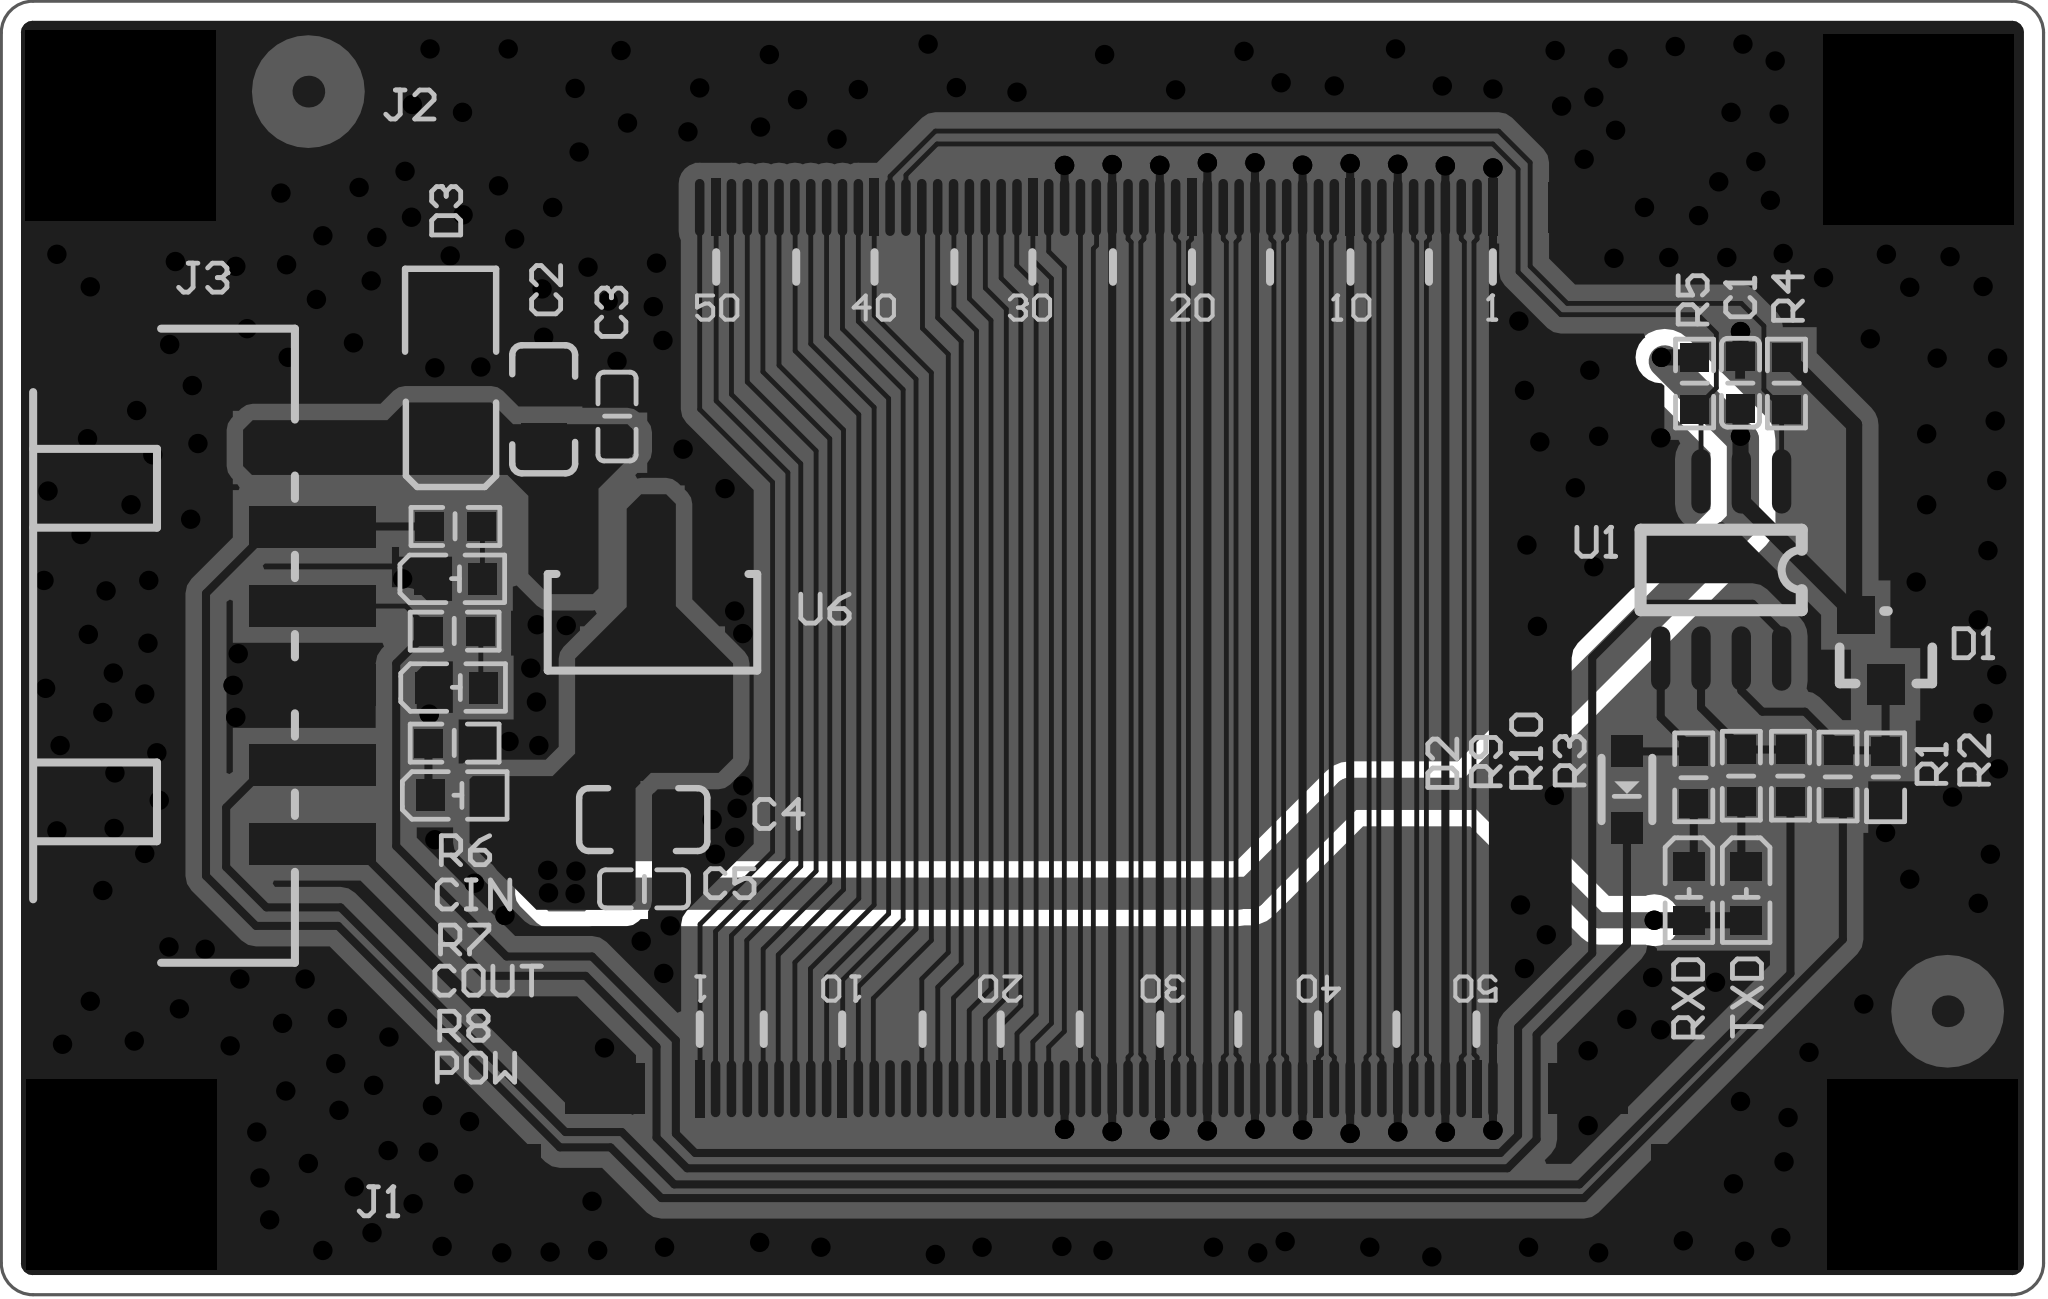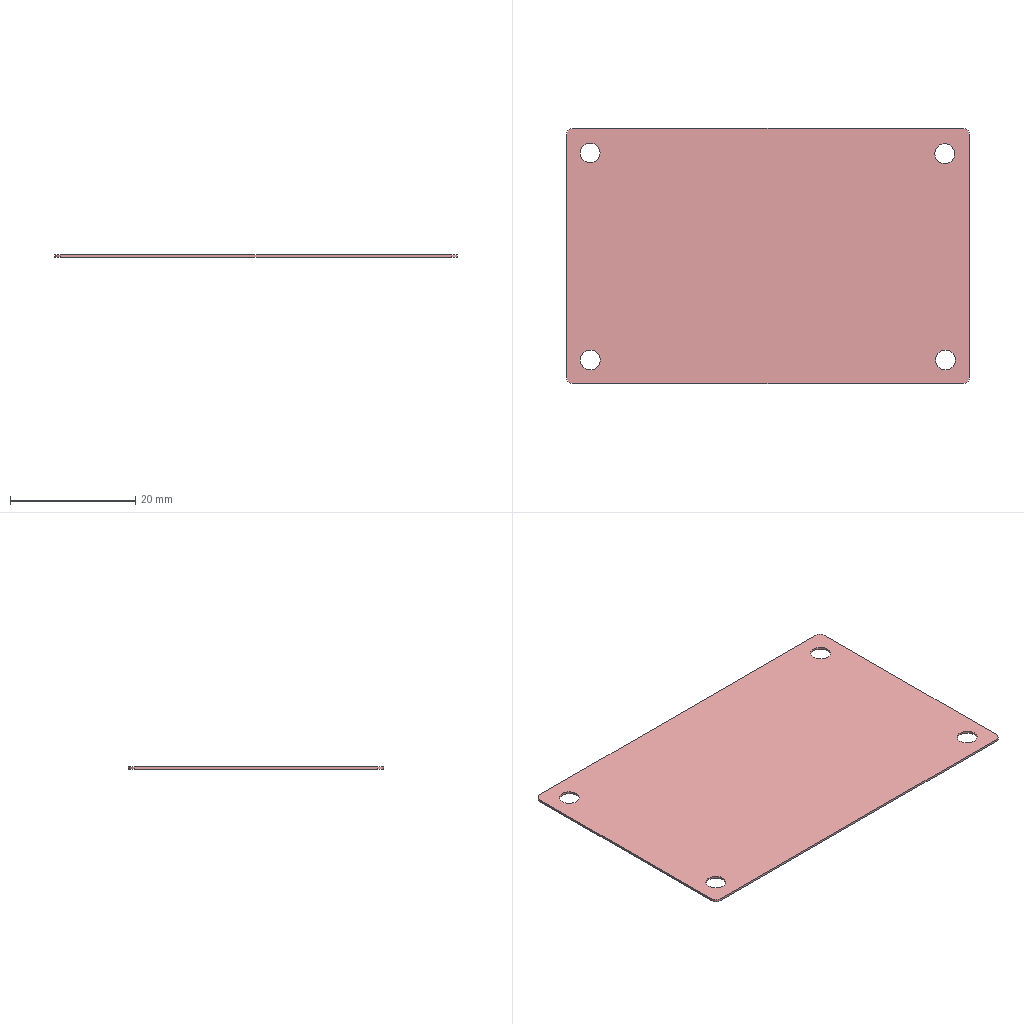Circuit board layout | Altium Designer | box 64.4 x 40.8 x 0.3 mm
Layer stack:
# Altium Designer layer stack of  (unit mm; dielectric type: 0 none, 1 core, 2 prepreg, 3 surface material)
index,name,kind,layer,copper_thickness_mm,dielectric_type,dielectric_thickness_mm,dielectric_material,dielectric_constant
0,Top Paste,other,,,,,,
1,Top Overlay,other,,,,,,
2,Top Solder,dielectric,,,3,0.0102,Solder Resist,3.5
3,Top Layer,copper,Top Layer,0.0356,,,,
4,Dielectric1,dielectric,,,1,0.254,FR-4,4.2
5,Bottom Layer,copper,Bottom Layer,0.0356,,,,
6,Bottom Solder,dielectric,,,3,0.0102,Solder Resist,3.5
7,Bottom Overlay,other,,,,,,
8,Bottom Paste,other,,,,,,
# drill layer pairs: low layer,high layer
drill_pair,Top Layer,Bottom Layer
Part placement:
Designator,Comment,Layer,Footprint,Center-X(mm),Center-Y(mm),Rotation
R6,4.7K,TopLayer,0603R,14.313,24.232,180
C1,0.1uf 50V,TopLayer,0603C,54.813,28.765,270
C2,10uF 16V,TopLayer,0805C,17.094,27.927,90
C3,0.1uf 50V,TopLayer,0603C,19.406,27.699,90
C4,10uF 16V,TopLayer,0805C,20.231,14.986,360
C5,0.1uf 50V,TopLayer,0603C,20.256,12.802,360
CIN,LED-RED,TopLayer,LED0603,14.314,22.581,270
COUT,LED-RED,TopLayer,LED0603,14.339,19.152,270
D2,1N5819,TopLayer,SOD-323,51.234,15.937,270
D3,SMAJ5.0A,TopLayer,1N5822,14.148,28.994,270
J1,FPC,TopLayer,FPC-0.5-51P,34.511,3.998,360
J2,FPC,TopLayer,FPC-0.5-51P,34.511,36.794,180
POW,LED-RED,TopLayer,LED0603,14.39,15.748,270
R1,1K,TopLayer,0603R,57.887,16.345,270
R2,4.7K,TopLayer,0603R,59.385,16.32,90
R3,100R,TopLayer,0603R,56.388,16.37,270
R4,4.7K,TopLayer,0603R,56.261,28.74,90
R5,4.7K,TopLayer,0603R,53.365,28.74,90
R7,4.7K,TopLayer,0603R,14.287,20.93,180
R8,4.7K,TopLayer,0603R,14.287,17.399,180
R9,4.7K,TopLayer,0603R,53.34,16.32,270
R10,4.7K,TopLayer,0603R,54.839,16.37,270
RXD,LED-RED,TopLayer,LED0603,53.188,12.661,180
TXD,LED-RED,TopLayer,LED0603,54.991,12.661,180
U6,1117-3.3,TopLayer,SOT-223,20.523,21.209,180
J3,CON8,TopLayer,CON6-Lay,6.304,20.471,270
U1,STC8G1K08,TopLayer,so-8,54.204,22.86,270
D1,BAV99,TopLayer,SOT-23,59.398,20.345,180
Pad and via stacks:
# Altium Designer via and pad stacks of  (unit mm). Each distinct definition once, with the count of objects using it.
# via: kind,start_layer,end_layer,hole_mm,diameter_mm,mode(0 simple;1 top-mid-bottom;2 full stack),diameter_per_layer,count,example_net
# pad: kind,layer,hole_mm,hole_type(0 round;1 square;2 slot),plating,top_size,top_shape(1 round;2 rect;3 octagon;9 rounded rect),mid_size,bottom_size,mode,footprint,size_per_layer,count,example
pad,Multi-Layer,3.2,0,plated,6x6,2,6x6,6x6,0,,,4,0
pad,Top Layer,0,0,plated,2.032x2.032,2,2.032x2.032,2.032x2.032,0,1N5822,,2,D3.1
pad,Top Layer,0,0,plated,2.4x4,2,2.4x4,2.4x4,0,CON6-Lay,,2,J3.8
pad,Top Layer,0,0,plated,1.3x4,2,1.3x4,1.3x4,0,CON6-Lay,,6,J3.6
pad,Top Layer,0,0,unplated,1x1,1,1x1,1x1,0,,,2,MARK
pad,Top Layer,0,0,plated,0.889x0.889,2,0.889x0.889,0.889x0.889,0,0603R,,20,R6.2
pad,Top Layer,0,0,plated,1.3x1.6,2,1.3x1.6,1.3x1.6,0,FPC-0.5-51P,,12,J2.52
pad,Top Layer,0,0,plated,2x2.5,2,2x2.5,2x2.5,0,FPC-0.5-51P,,4,J2.52
pad,Top Layer,0,0,plated,1.6x2.5,2,1.6x2.5,1.6x2.5,0,FPC-0.5-51P,,4,J2.52
pad,Top Layer,0,0,plated,0.3x1.8,1,0.3x1.8,0.3x1.8,0,FPC-0.5-51P,,90,J2.51
pad,Top Layer,0,0,plated,0.3x1.8,2,0.3x1.8,0.3x1.8,0,FPC-0.5-51P,,12,J2.50
pad,Top Layer,0,0,plated,0.889x0.889,2,0.889x0.889,0.889x0.889,0,0603C,,6,C1.2
pad,Top Layer,0,0,plated,1x0.8999,2,1x0.8999,1x0.8999,0,LED0603,,10,CIN.1
pad,Top Layer,0,0,plated,1.016x2.794,2,1.016x2.794,1.016x2.794,0,SOT-223,,3,U6.3
pad,Top Layer,0,0,plated,3.556x3.556,2,3.556x3.556,3.556x3.556,0,SOT-223,,1,U6.2
pad,Top Layer,0,0,plated,1.168x1.168,2,1.168x1.168,1.168x1.168,0,SOT-23,,2,D1.1
pad,Top Layer,0,0,plated,1.168x1.27,2,1.168x1.27,1.168x1.27,0,SOT-23,,1,D1.3
pad,Top Layer,0,0,plated,1x1,2,1x1,1x1,0,SOD-323,,2,D2.1
pad,Top Layer,0,0,plated,1.321x1.422,2,1.321x1.422,1.321x1.422,0,0805C,,4,C4.1
pad,Top Layer,0,0,plated,2.032x0.6096,1,2.032x0.6096,2.032x0.6096,0,so-8,,8,U1.5
via,Top Layer,Bottom Layer,0.3048,0.6096,0,,259,GND
Copper pours:
name,layer,net,type(0 solid;1 hatched;2 none)
BottomLayer-No Net,Top Layer,GND,0
BottomLayer-No Net,Top Layer,VCC_3.3V,0
BottomLayer-No Net,Top Layer,VCC_5V,0
BottomLayer-No Net,Bottom Layer,GND,0
BottomLayer-No Net,Bottom Layer,VCC_3.3V,0
Design rules, without the lines most boards share:
# Altium Designer design rules of  (exported by Altium Designer, unit mm)
# columns: name | kind | enabled | priority | scope1 | scope2 | descriptor | typed fields (field=value)
Clearance_1 | 0 | enabled | 1 | haspad('free-mark') | All | Clearance Constraint (Gap=50mil) (haspad('free-mark')),(All) | gap=1.27
PolygonConnect_FULL | 20 | enabled | 1 | InPadClass('FULL') Or ISVIA | All | Polygon Connect Rule(Direct Connect )(Conductor Width=10mil) (Relief Angle=90 Angle) (Entries=4) (Air Gap Width=10mil) (InPadClass('FULL') Or ISVIA),(All) | connect_style(0=relief,1=direct,2=none)=1 relief_conductor_width=0.254 relief_entries=4
Clearance_inpoly | 0 | enabled | 2 | inpolygon | All | Clearance Constraint (Gap=20mil) (inpolygon),(All) | gap=0.508
SilkToSilkClearance | 55 | disabled | 1 | All | All | Silk to Silk (Clearance=10mil) (Disabled)(All),(All) |
SilkToSolderMaskClearance | 54 | disabled | 1 | IsPad | All | Silk To Solder Mask (Clearance=10mil) (Disabled)(IsPad),(All) |
MinimumSolderMaskSliver | 53 | disabled | 1 | All | All | Minimum Solder Mask Sliver (Gap=10mil) (Disabled)(All),(All) |
HoleToHoleClearance | 52 | enabled | 1 | All | All | Hole To Hole Clearance (Gap=10mil) (All),(All) | gap=0.254
DiffPairsRouting | 51 | enabled | 1 | All | All | Differential Pairs Uncoupled Length using the Gap Constraints (Min=6mil) (Max=40mil) (Prefered=6mil)  and Width Constraints (Min=15mil) (Max=15mil) (Prefered=15mil) (All) |
HoleSize | 42 | disabled | 1 | All | All | Hole Size Constraint (Min=1mil) (Max=100mil) (Disabled)(All) |
Height | 50 | disabled | 1 | All | All | Height Constraint (Min=0mil) (Max=1000mil) (Prefered=500mil) (Disabled)(All) | min_height=0 max_height=25.4
ComponentClearance | 24 | disabled | 1 | All | All | Component Clearance Constraint ( Horizontal Gap = 10mil, Vertical Gap = 10mil ) (Disabled)(All),(All)  | gap=0.254
SolderMaskExpansion | 13 | disabled | 1 | All | All | Solder Mask Expansion (Expansion =4mil) (Disabled)(All) | expansion=0.1016
PasteMaskExpansion | 14 | disabled | 1 | All | All | Paste Mask Expansion (Expansion =0mil) (Disabled)(All) | expansion=0
RoutingVias | 11 | enabled | 1 | All | All | Routing Via (MinHoleWidth=12mil) (MaxHoleWidth=12mil) (PreferredHoleWidth=12mil) (MinWidth=24mil) (MaxWidth=24mil) (PreferedWidth=24mil) (All) | via_min_hole=0.3048 via_max_hole=0.3048 via_preferred_diameter=0.6096 via_preferred_hole=0.3048
Width | 2 | enabled | 1 | All | All | Width Constraint (Min=6mil) (Max=100mil) (Preferred=6mil) (All) |
PolygonConnect | 20 | enabled | 2 | All | All | Polygon Connect Rule(Direct Connect )(Conductor Width=10mil) (Relief Angle=90 Angle) (Entries=4) (Air Gap Width=10mil) (All),(All) | connect_style(0=relief,1=direct,2=none)=1 relief_conductor_width=0.254 relief_entries=4
PlaneConnect | 6 | enabled | 1 | All | All | Power Plane Connect Rule(Relief Connect )(Expansion=20mil) (Conductor Width=10mil) (Air Gap=10mil) (Entries=4) (All) | relief_conductor_width=0.254 relief_entries=4 relief_expansion=0.508
Clearance | 0 | enabled | 3 | All | All | Clearance Constraint (Gap=6mil) (All),(All) | gap=0.1524
Classes set for this board:
# Altium Designer classes of  (member kind: 0 net, 1 component, 2 from-to, 3 pad, 4 layer, 5 differential pair, 6 design channel, 7 polygon, 8 structure, 9 xSignal)
# columns: class name | member kind | superclass | members
FULL | 3 | no |
L3870_V1 | 1 | no | C1; C2; C3; C4; C5; CIN; COUT; D1; D2; D3; J1; J2; J3; POW; R1; R2; R3; R4; R5; R6; R7; R8; R9; R10; RXD; TXD; U1; U6; J3; U1; D1;